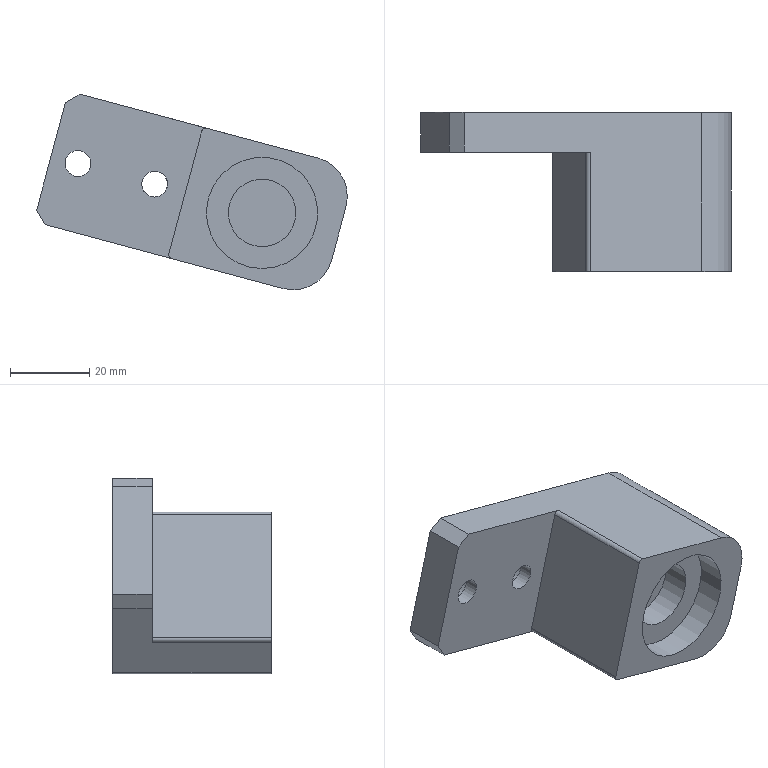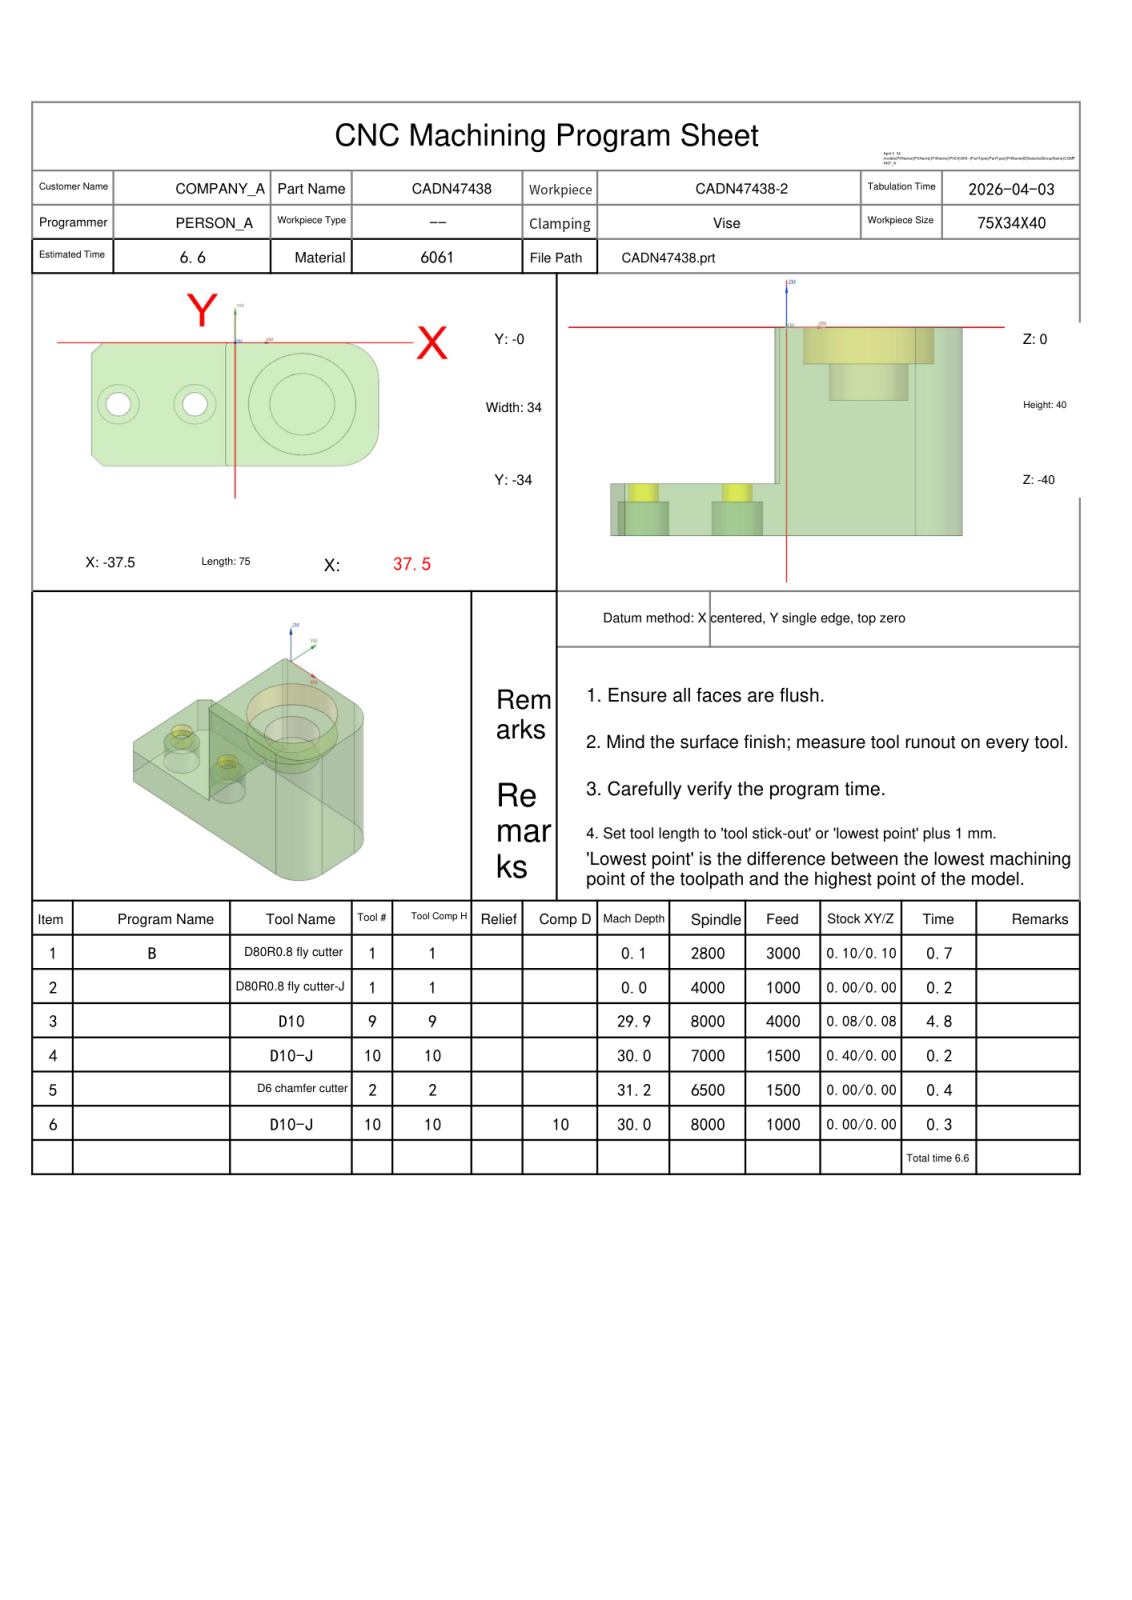NC program | NX | posted by the shop | part box 78.22 x 40 x 49.229 mm
Lines 2493 to 2756 of 2756:
N4 T10 M06
(D10-J  D=10. R=0. H=10 ce=0.40 di=0.00)
G00 G90 G54 X-43.907 Y-34.014 M03 S7000
G43 H10 Z14.5
M08
Z-28.5
G01 Z-30. F1500.
X-39.9
G03 X-37.9 Y-32.014 I0.0 J2.
G01 Y-2.4
G02 X-37.607 Y-1.693 I1. J0.0
G01 X-35.207 Y.707
G02 X-34.5 Y1. I.707 J-.707
G01 X-33.781
G02 X-32.881 Y.1 I0.0 J-.9
G01 X-32.882 Y.07
G03 X-32.9 Y-.999 I31.382 J-1.07
G01 Y-33.
G03 X-32.883 Y-34.033 I31.4 J0.0
X-31.884 Y-35. I.999 J.033
G01 X-28.777
G03 X-27.878 Y-34.1 I0.0 J.9
G01 X-27.879 Y-34.064
G02 X-27.9 Y-33. I26.379 J1.064
G01 Y-.999
G02 X-27.88 Y.04 I26.4 J-.001
X-26.881 Y1. I.999 J-.04
G01 X-23.772
G02 X-22.873 Y.1 I0.0 J-.9
G01 X-22.874 Y.056
G03 X-22.9 Y-.999 I21.374 J-1.056
G01 Y-33.
G03 X-22.874 Y-34.049 I21.4 J0.0
X-21.876 Y-35. I.999 J.049
G01 X-18.765
G03 X-17.865 Y-34.1 I0.0 J.9
G01 X-17.867 Y-34.043
G02 X-17.9 Y-33. I16.367 J1.043
G01 Y-1.
G02 X-17.865 Y.065 I16.4 J0.0
X-16.868 Y1. I.998 J-.065
G01 X-13.64
G02 X-12.841 Y.2 I0.0 J-.8
G01 X-12.845 Y.122
G03 X-12.9 Y-1. I11.345 J-1.122
G01 Y-33.
G03 X-12.819 Y-34.36 I11.4 J0.0
X-12.136 Y-35.191 I.993 J.12
G01 X-8.839 Y-36.263
G03 X-8.529 Y-36.313 I.309 J.951
X-7.529 Y-35.313 I0.0 J1.
X-7.579 Y-35. I-1. J0.0
G02 X-7.9 Y-33. I6.079 J2.
G01 Y-1.
G02 X-7.579 Y1. I6.4 J0.0
G03 X-7.479 Y1.625 I-1.9 J.625
X-8.854 Y3.525 I-2. J0.0
G01 Y7.
Z-28.5
G00 Z14.5
G91 G28 Z0.0
M05
M09
G91 G28 Z0.0
M01
N5 T02 M06
(D6 chamfer cutter  D=6. R=0. H=02 ce=0.00 di=0.00)
G00 G90 G54 X-3.427 Y-17.386 M03 S6500
G43 H02 Z20.
M08
Z.472
G01 Z-1.199 F1500.
G03 X-3.227 Y-17.1 I-1.532 J1.286
G01 X-3.197 Y-17.054
X-3.2 Y-17.
Y-1.
G02 X-1.5 Y.7 I1.7 J0.0
G01 X27.5
G02 X38.2 Y-10. I0.0 J-10.7
G01 Y-24.
G02 X27.5 Y-34.7 I-10.7 J0.0
G01 X-1.5
G02 X-3.2 Y-33. I0.0 J1.7
G01 Y-17.
X-3.197 Y-16.946
X-3.227 Y-16.9
G03 X-3.427 Y-16.614 I-1.732 J-1.
G01 Z.472
G00 Z10.
X20.512 Y-29.763
Z.494
G01 Z-1.199
G03 X20.844 Y-29.87 I.777 J1.843
G01 X20.896 Y-29.885
X20.947 Y-29.866
G03 X30.82 Y-17. I-3.447 J12.866
X17.5 Y-3.68 I-13.32 J0.0
X4.18 Y-17. I0.0 J-13.32
X17.5 Y-30.32 I13.32 J0.0
X20.947 Y-29.866 I0.0 J13.32
G01 X21.001 Y-29.857
X21.039 Y-29.818
G03 X21.273 Y-29.559 I-1.36 J1.466
G01 Z.494
G00 Z10.
X15.918 Y-9.564
Z-6.495
G01 Z-8.199
G03 X15.585 Y-9.461 I-.758 J-1.851
G01 X15.532 Y-9.447
X15.481 Y-9.466
G03 X9.7 Y-17. I2.019 J-7.534
X17.5 Y-24.8 I7.8 J0.0
X25.3 Y-17. I0.0 J7.8
X17.5 Y-9.2 I-7.8 J0.0
X15.481 Y-9.466 I0.0 J-7.8
G01 X15.427 Y-9.475
X15.389 Y-9.513
G03 X15.153 Y-9.769 I1.345 J-1.48
G01 Z-6.492
G00 Z10.
X-5.316 Y-34.768
Z-1.812
G01 Z-31.199
X-5.402 Y-34.708
X-5.432 Y-34.7
X-34.5
X-34.681 Y-34.676
X-34.85 Y-34.606
X-34.995 Y-34.495
X-37.995 Y-31.495
X-38.106 Y-31.35
X-38.176 Y-31.181
X-38.2 Y-31.
Y-3.
X-38.176 Y-2.819
X-38.106 Y-2.65
X-37.995 Y-2.505
X-34.995 Y.495
X-34.85 Y.606
X-34.681 Y.676
X-34.5 Y.7
X-5.432
X-5.402 Y.708
X-5.316 Y.768
Z-1.812
G00 Z10.
X-30.28 Y-19.382
Z-29.45
G01 Z-31.199
G03 X-29.943 Y-19.472 I.684 J1.879
G01 X-29.89 Y-19.484
X-29.84 Y-19.463
G03 X-27.95 Y-17. I-.66 J2.463
X-30.5 Y-14.45 I-2.55 J0.0
X-33.05 Y-17. I0.0 J-2.55
X-30.5 Y-19.55 I2.55 J0.0
X-29.84 Y-19.463 I0.0 J2.55
G01 X-29.786 Y-19.456
X-29.746 Y-19.419
G03 X-29.5 Y-19.173 I-1.286 J1.532
G01 Z-29.453
G00 Z10.
X-10.28 Y-19.382
Z-29.45
G01 Z-31.199
G03 X-9.943 Y-19.472 I.684 J1.879
G01 X-9.89 Y-19.484
X-9.84 Y-19.463
G03 X-7.95 Y-17. I-.66 J2.463
X-10.5 Y-14.45 I-2.55 J0.0
X-13.05 Y-17. I0.0 J-2.55
X-10.5 Y-19.55 I2.55 J0.0
X-9.84 Y-19.463 I0.0 J2.55
G01 X-9.786 Y-19.456
X-9.746 Y-19.419
G03 X-9.5 Y-19.173 I-1.286 J1.532
G01 Z-29.453
G00 Z20.
G91 G28 Z0.0
M05
M09
G91 G28 Z0.0
M01
N6 T10 M06
(D10-J  D=10. R=0. H=10 ce=0.00 di=0.00)
G00 G90 G54 X16.342 Y-18.473 M03 S8000
G43 H10 Z14.5
M08
Z-12.5
G01 Z-14. F600.
G41 D10
X16.569 Y-19.32
G03 X18.018 Y-20.432 I1.449 J.388
X18.406 Y-20.381 I0.0 J1.5
X21. Y-17. I-.906 J3.381
X17.5 Y-13.5 I-3.5 J0.0
X14. Y-17. I0.0 J-3.5
X17.5 Y-20.5 I3.5 J0.0
X18.406 Y-20.381 I0.0 J3.5
X18.785 Y-20.255 I-.906 J3.381
X19.735 Y-18.86 I-.551 J1.395
X19.63 Y-18.309 I-1.5 J0.0
G01 X19.381 Y-17.679
G40 X19.308 Y-17.493
Z-12.5
G00 Z14.5
G00 G90 X17.907 Y-24.313 M03 S8000
Z14.5
Z-5.5
G01 Z-7. F1000.
G41 D10
X17.997 Y-24.652
G03 X19.446 Y-25.764 I1.449 J.388
X19.835 Y-25.713 I0.0 J1.5
X26.52 Y-17. I-2.335 J8.713
X17.5 Y-7.98 I-9.02 J0.0
X8.48 Y-17. I0.0 J-9.02
X17.5 Y-26.02 I9.02 J0.0
X19.835 Y-25.713 I0.0 J9.02
X20.218 Y-25.601 I-2.335 J8.713
X21.266 Y-24.17 I-.452 J1.43
X21.197 Y-23.718 I-1.5 J0.0
G01 X21.151 Y-23.574
G40 X21.091 Y-23.383
Z-5.5
G00 Z14.5
G00 G90 X.247 Y-41.2 M03 S8000
Z14.5
Z-14.
G01 Z-15. F1000.
G41 D10
Y-41.
Y-40.996
G03 X-1.69 Y-38.997 I-2. J0.0
G02 X-7.5 Y-33. I.19 J5.997
G01 Y-1.
G02 X-1.69 Y4.997 I6. J0.0
G03 X.247 Y6.996 I-.063 J1.999
G01 Y7.
G40 Y7.2
Z-14.
G00 Z14.5
Y-41.2
Z-29.
G01 Z-30.
G41 D10
Y-41.
Y-40.996
G03 X-1.69 Y-38.997 I-2. J0.0
G02 X-7.5 Y-33. I.19 J5.997
G01 Y-1.
G02 X-1.69 Y4.997 I6. J0.0
G03 X.247 Y6.996 I-.063 J1.999
G01 Y7.
G40 Y7.2
Z-29.
G00 Z14.5
M05
M09
G91 G28 Z0.0
G91 G28 Y0.0
M30
%